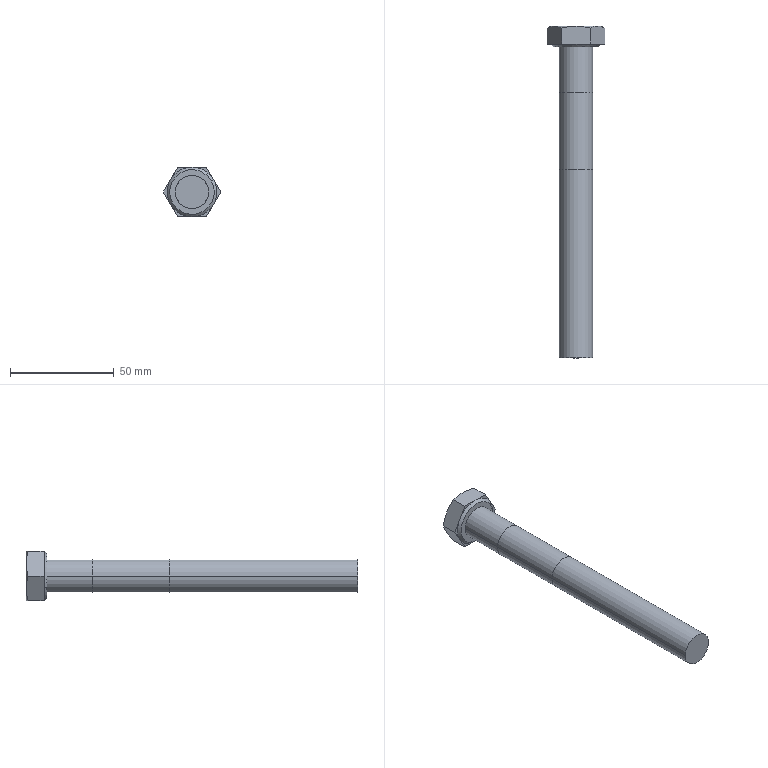Part | NX | features BREP 2, DELETE FACE 1, OFFSET_REGION 1 | 1 solid | 29 faces | box 27.713 x 160 x 24 mm | volume 38117 mm3 | plane 17 | cone 8 | cylinder 4 | commonest cylinder face diameters 13.835 x2 16 x2